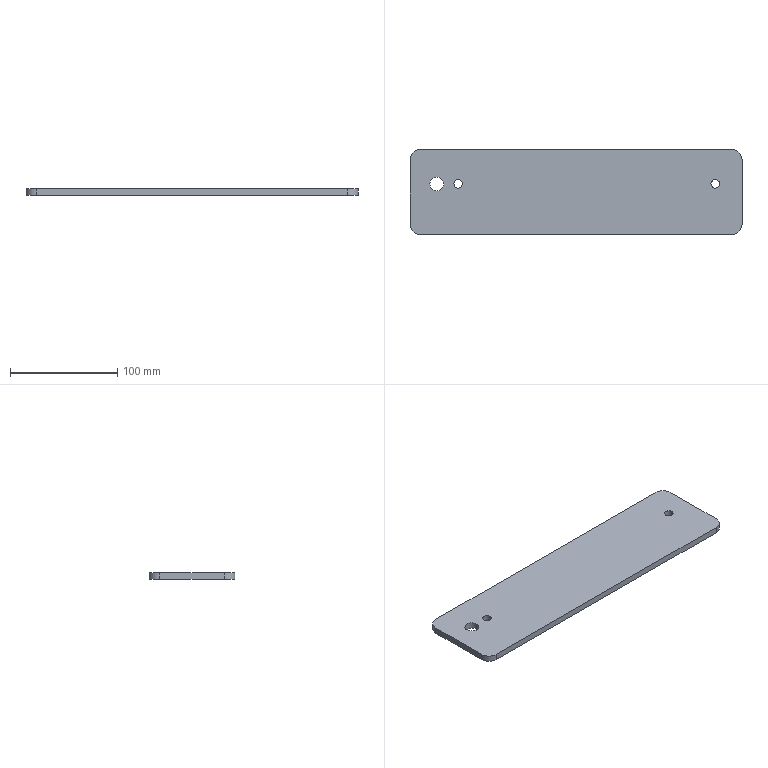Part | SolidWorks | features FlatPattern 1, SMBaseFlange 1, SheetMetal 1 | 1 solid | 16 faces | box 310 x 80 x 6 mm | volume 146885 mm3 | cylinder 10 | plane 6 | commonest cylinder face diameters 8 x4 20 x4 13 x2
STEP:
#1=CARTESIAN_POINT('',(-1194.,-927.5,6.));
#2=VERTEX_POINT('',#1);
#3=CARTESIAN_POINT('',(-1186.,-927.5,6.));
#4=VERTEX_POINT('',#3);
#5=CARTESIAN_POINT('',(-1190.,-927.5,6.));
#6=DIRECTION('',(0.,0.,1.));
#7=DIRECTION('',(1.,0.,0.));
#8=AXIS2_PLACEMENT_3D('',#5,#6,#7);
#9=CIRCLE('',#8,4.);
#10=EDGE_CURVE('',#2,#4,#9,.T.);
#11=ORIENTED_EDGE('',*,*,#10,.T.);
#12=CARTESIAN_POINT('',(-1186.,-927.5,0.));
#13=VERTEX_POINT('',#12);
#14=CARTESIAN_POINT('',(-1186.,-927.5,6.));
#15=DIRECTION('',(0.,0.,-1.));
#16=VECTOR('',#15,1000.);
#17=LINE('',#14,#16);
#18=EDGE_CURVE('',#4,#13,#17,.T.);
#19=ORIENTED_EDGE('',*,*,#18,.T.);
#20=CARTESIAN_POINT('',(-1194.,-927.5,0.));
#21=VERTEX_POINT('',#20);
#22=CARTESIAN_POINT('',(-1190.,-927.5,0.));
#23=DIRECTION('',(0.,0.,1.));
#24=DIRECTION('',(1.,0.,0.));
#25=AXIS2_PLACEMENT_3D('',#22,#23,#24);
#26=CIRCLE('',#25,4.);
#27=EDGE_CURVE('',#21,#13,#26,.T.);
#28=ORIENTED_EDGE('',*,*,#27,.F.);
#29=CARTESIAN_POINT('',(-1194.,-927.5,6.));
#30=DIRECTION('',(0.,0.,-1.));
#31=VECTOR('',#30,1000.);
#32=LINE('',#29,#31);
#33=EDGE_CURVE('',#2,#21,#32,.T.);
#34=ORIENTED_EDGE('',*,*,#33,.F.);
#35=EDGE_LOOP('',(#11,#19,#28,#34));
#36=FACE_OUTER_BOUND('',#35,.T.);
#37=CARTESIAN_POINT('',(-1190.,-927.5,6.));
#38=DIRECTION('',(0.,0.,-1.));
#39=DIRECTION('',(-1.,0.,0.));
#40=AXIS2_PLACEMENT_3D('',#37,#38,#39);
#41=CYLINDRICAL_SURFACE('',#40,4.);
#42=ADVANCED_FACE('',(#36),#41,.F.);
#43=CARTESIAN_POINT('',(-1434.,-927.5,6.));
#44=VERTEX_POINT('',#43);
#45=CARTESIAN_POINT('',(-1426.,-927.5,6.));
#46=VERTEX_POINT('',#45);
#47=CARTESIAN_POINT('',(-1430.,-927.5,6.));
#48=DIRECTION('',(0.,0.,1.));
#49=DIRECTION('',(1.,0.,0.));
#50=AXIS2_PLACEMENT_3D('',#47,#48,#49);
#51=CIRCLE('',#50,4.);
#52=EDGE_CURVE('',#44,#46,#51,.T.);
#53=ORIENTED_EDGE('',*,*,#52,.T.);
#54=CARTESIAN_POINT('',(-1426.,-927.5,0.));
#55=VERTEX_POINT('',#54);
#56=CARTESIAN_POINT('',(-1426.,-927.5,6.));
#57=DIRECTION('',(0.,0.,-1.));
#58=VECTOR('',#57,1000.);
#59=LINE('',#56,#58);
#60=EDGE_CURVE('',#46,#55,#59,.T.);
#61=ORIENTED_EDGE('',*,*,#60,.T.);
#62=CARTESIAN_POINT('',(-1434.,-927.5,0.));
#63=VERTEX_POINT('',#62);
#64=CARTESIAN_POINT('',(-1430.,-927.5,0.));
#65=DIRECTION('',(0.,0.,1.));
#66=DIRECTION('',(1.,0.,0.));
#67=AXIS2_PLACEMENT_3D('',#64,#65,#66);
#68=CIRCLE('',#67,4.);
#69=EDGE_CURVE('',#63,#55,#68,.T.);
#70=ORIENTED_EDGE('',*,*,#69,.F.);
#71=CARTESIAN_POINT('',(-1434.,-927.5,6.));
#72=DIRECTION('',(0.,0.,-1.));
#73=VECTOR('',#72,1000.);
#74=LINE('',#71,#73);
#75=EDGE_CURVE('',#44,#63,#74,.T.);
#76=ORIENTED_EDGE('',*,*,#75,.F.);
#77=EDGE_LOOP('',(#53,#61,#70,#76));
#78=FACE_OUTER_BOUND('',#77,.T.);
#79=CARTESIAN_POINT('',(-1430.,-927.5,6.));
#80=DIRECTION('',(0.,0.,-1.));
#81=DIRECTION('',(-1.,0.,0.));
#82=AXIS2_PLACEMENT_3D('',#79,#80,#81);
#83=CYLINDRICAL_SURFACE('',#82,4.);
#84=ADVANCED_FACE('',(#78),#83,.F.);
#85=CARTESIAN_POINT('',(-1456.5,-927.5,6.));
#86=VERTEX_POINT('',#85);
#87=CARTESIAN_POINT('',(-1443.5,-927.5,6.));
#88=VERTEX_POINT('',#87);
#89=CARTESIAN_POINT('',(-1450.,-927.5,6.));
#90=DIRECTION('',(0.,0.,1.));
#91=DIRECTION('',(1.,0.,0.));
#92=AXIS2_PLACEMENT_3D('',#89,#90,#91);
#93=CIRCLE('',#92,6.5);
#94=EDGE_CURVE('',#86,#88,#93,.T.);
#95=ORIENTED_EDGE('',*,*,#94,.T.);
#96=CARTESIAN_POINT('',(-1443.5,-927.5,0.));
#97=VERTEX_POINT('',#96);
#98=CARTESIAN_POINT('',(-1443.5,-927.5,6.));
#99=DIRECTION('',(0.,0.,-1.));
#100=VECTOR('',#99,1000.);
#101=LINE('',#98,#100);
#102=EDGE_CURVE('',#88,#97,#101,.T.);
#103=ORIENTED_EDGE('',*,*,#102,.T.);
#104=CARTESIAN_POINT('',(-1456.5,-927.5,0.));
#105=VERTEX_POINT('',#104);
#106=CARTESIAN_POINT('',(-1450.,-927.5,0.));
#107=DIRECTION('',(0.,0.,1.));
#108=DIRECTION('',(1.,0.,0.));
#109=AXIS2_PLACEMENT_3D('',#106,#107,#108);
#110=CIRCLE('',#109,6.5);
#111=EDGE_CURVE('',#105,#97,#110,.T.);
#112=ORIENTED_EDGE('',*,*,#111,.F.);
#113=CARTESIAN_POINT('',(-1456.5,-927.5,6.));
#114=DIRECTION('',(0.,0.,-1.));
#115=VECTOR('',#114,1000.);
#116=LINE('',#113,#115);
#117=EDGE_CURVE('',#86,#105,#116,.T.);
#118=ORIENTED_EDGE('',*,*,#117,.F.);
#119=EDGE_LOOP('',(#95,#103,#112,#118));
#120=FACE_OUTER_BOUND('',#119,.T.);
#121=CARTESIAN_POINT('',(-1450.,-927.5,6.));
#122=DIRECTION('',(0.,0.,-1.));
#123=DIRECTION('',(-1.,0.,0.));
#124=AXIS2_PLACEMENT_3D('',#121,#122,#123);
#125=CYLINDRICAL_SURFACE('',#124,6.5);
#126=ADVANCED_FACE('',(#120),#125,.F.);
#127=CARTESIAN_POINT('',(-1165.,-905.,6.));
#128=VERTEX_POINT('',#127);
#129=CARTESIAN_POINT('',(-1175.,-895.,6.));
#130=VERTEX_POINT('',#129);
#131=CARTESIAN_POINT('',(-1175.,-905.,6.));
#132=DIRECTION('',(0.,0.,1.));
#133=DIRECTION('',(-1.,0.,0.));
#134=AXIS2_PLACEMENT_3D('',#131,#132,#133);
#135=CIRCLE('',#134,10.);
#136=EDGE_CURVE('',#128,#130,#135,.T.);
#137=ORIENTED_EDGE('',*,*,#136,.T.);
#138=CARTESIAN_POINT('',(-1465.,-895.,6.));
#139=VERTEX_POINT('',#138);
#140=CARTESIAN_POINT('',(-1465.,-895.,6.));
#141=DIRECTION('',(-1.,0.,0.));
#142=VECTOR('',#141,1000.);
#143=LINE('',#140,#142);
#144=EDGE_CURVE('',#130,#139,#143,.T.);
#145=ORIENTED_EDGE('',*,*,#144,.T.);
#146=CARTESIAN_POINT('',(-1475.,-905.,6.));
#147=VERTEX_POINT('',#146);
#148=CARTESIAN_POINT('',(-1465.,-905.,6.));
#149=DIRECTION('',(0.,0.,1.));
#150=DIRECTION('',(-1.,0.,0.));
#151=AXIS2_PLACEMENT_3D('',#148,#149,#150);
#152=CIRCLE('',#151,10.);
#153=EDGE_CURVE('',#139,#147,#152,.T.);
#154=ORIENTED_EDGE('',*,*,#153,.T.);
#155=CARTESIAN_POINT('',(-1475.,-965.,6.));
#156=VERTEX_POINT('',#155);
#157=CARTESIAN_POINT('',(-1475.,-965.,6.));
#158=DIRECTION('',(0.,-1.,0.));
#159=VECTOR('',#158,1000.);
#160=LINE('',#157,#159);
#161=EDGE_CURVE('',#147,#156,#160,.T.);
#162=ORIENTED_EDGE('',*,*,#161,.T.);
#163=CARTESIAN_POINT('',(-1465.,-975.,6.));
#164=VERTEX_POINT('',#163);
#165=CARTESIAN_POINT('',(-1465.,-965.,6.));
#166=DIRECTION('',(0.,0.,1.));
#167=DIRECTION('',(-1.,0.,0.));
#168=AXIS2_PLACEMENT_3D('',#165,#166,#167);
#169=CIRCLE('',#168,10.);
#170=EDGE_CURVE('',#156,#164,#169,.T.);
#171=ORIENTED_EDGE('',*,*,#170,.T.);
#172=CARTESIAN_POINT('',(-1175.,-975.,6.));
#173=VERTEX_POINT('',#172);
#174=CARTESIAN_POINT('',(-1465.,-975.,6.));
#175=DIRECTION('',(1.,0.,0.));
#176=VECTOR('',#175,1000.);
#177=LINE('',#174,#176);
#178=EDGE_CURVE('',#164,#173,#177,.T.);
#179=ORIENTED_EDGE('',*,*,#178,.T.);
#180=CARTESIAN_POINT('',(-1165.,-965.,6.));
#181=VERTEX_POINT('',#180);
#182=CARTESIAN_POINT('',(-1175.,-965.,6.));
#183=DIRECTION('',(0.,0.,1.));
#184=DIRECTION('',(1.,0.,0.));
#185=AXIS2_PLACEMENT_3D('',#182,#183,#184);
#186=CIRCLE('',#185,10.);
#187=EDGE_CURVE('',#173,#181,#186,.T.);
#188=ORIENTED_EDGE('',*,*,#187,.T.);
#189=CARTESIAN_POINT('',(-1165.,-965.,6.));
#190=DIRECTION('',(0.,1.,0.));
#191=VECTOR('',#190,1000.);
#192=LINE('',#189,#191);
#193=EDGE_CURVE('',#181,#128,#192,.T.);
#194=ORIENTED_EDGE('',*,*,#193,.T.);
#195=EDGE_LOOP('',(#137,#145,#154,#162,#171,#179,#188,#194));
#196=FACE_OUTER_BOUND('',#195,.T.);
#197=ORIENTED_EDGE('',*,*,#94,.F.);
#198=CARTESIAN_POINT('',(-1450.,-927.5,6.));
#199=DIRECTION('',(0.,0.,1.));
#200=DIRECTION('',(1.,0.,0.));
#201=AXIS2_PLACEMENT_3D('',#198,#199,#200);
#202=CIRCLE('',#201,6.5);
#203=EDGE_CURVE('',#88,#86,#202,.T.);
#204=ORIENTED_EDGE('',*,*,#203,.F.);
#205=EDGE_LOOP('',(#197,#204));
#206=FACE_BOUND('',#205,.T.);
#207=ORIENTED_EDGE('',*,*,#52,.F.);
#208=CARTESIAN_POINT('',(-1430.,-927.5,6.));
#209=DIRECTION('',(0.,0.,1.));
#210=DIRECTION('',(1.,0.,0.));
#211=AXIS2_PLACEMENT_3D('',#208,#209,#210);
#212=CIRCLE('',#211,4.);
#213=EDGE_CURVE('',#46,#44,#212,.T.);
#214=ORIENTED_EDGE('',*,*,#213,.F.);
#215=EDGE_LOOP('',(#207,#214));
#216=FACE_BOUND('',#215,.T.);
#217=ORIENTED_EDGE('',*,*,#10,.F.);
#218=CARTESIAN_POINT('',(-1190.,-927.5,6.));
#219=DIRECTION('',(0.,0.,1.));
#220=DIRECTION('',(1.,0.,0.));
#221=AXIS2_PLACEMENT_3D('',#218,#219,#220);
#222=CIRCLE('',#221,4.);
#223=EDGE_CURVE('',#4,#2,#222,.T.);
#224=ORIENTED_EDGE('',*,*,#223,.F.);
#225=EDGE_LOOP('',(#217,#224));
#226=FACE_BOUND('',#225,.T.);
#227=CARTESIAN_POINT('',(-1175.,-905.,6.));
#228=DIRECTION('',(0.,0.,-1.));
#229=DIRECTION('',(-1.,0.,0.));
#230=AXIS2_PLACEMENT_3D('',#227,#228,#229);
#231=PLANE('',#230);
#232=ADVANCED_FACE('',(#196,#206,#216,#226),#231,.F.);
#233=ORIENTED_EDGE('',*,*,#69,.T.);
#234=CARTESIAN_POINT('',(-1430.,-927.5,0.));
#235=DIRECTION('',(0.,0.,1.));
#236=DIRECTION('',(1.,0.,0.));
#237=AXIS2_PLACEMENT_3D('',#234,#235,#236);
#238=CIRCLE('',#237,4.);
#239=EDGE_CURVE('',#55,#63,#238,.T.);
#240=ORIENTED_EDGE('',*,*,#239,.T.);
#241=EDGE_LOOP('',(#233,#240));
#242=FACE_BOUND('',#241,.T.);
#243=CARTESIAN_POINT('',(-1165.,-905.,0.));
#244=VERTEX_POINT('',#243);
#245=CARTESIAN_POINT('',(-1175.,-895.,0.));
#246=VERTEX_POINT('',#245);
#247=CARTESIAN_POINT('',(-1175.,-905.,0.));
#248=DIRECTION('',(0.,0.,1.));
#249=DIRECTION('',(-1.,0.,0.));
#250=AXIS2_PLACEMENT_3D('',#247,#248,#249);
#251=CIRCLE('',#250,10.);
#252=EDGE_CURVE('',#244,#246,#251,.T.);
#253=ORIENTED_EDGE('',*,*,#252,.F.);
#254=CARTESIAN_POINT('',(-1165.,-965.,0.));
#255=VERTEX_POINT('',#254);
#256=CARTESIAN_POINT('',(-1165.,-965.,0.));
#257=DIRECTION('',(0.,1.,0.));
#258=VECTOR('',#257,1000.);
#259=LINE('',#256,#258);
#260=EDGE_CURVE('',#255,#244,#259,.T.);
#261=ORIENTED_EDGE('',*,*,#260,.F.);
#262=CARTESIAN_POINT('',(-1175.,-975.,0.));
#263=VERTEX_POINT('',#262);
#264=CARTESIAN_POINT('',(-1175.,-965.,0.));
#265=DIRECTION('',(0.,0.,1.));
#266=DIRECTION('',(1.,0.,0.));
#267=AXIS2_PLACEMENT_3D('',#264,#265,#266);
#268=CIRCLE('',#267,10.);
#269=EDGE_CURVE('',#263,#255,#268,.T.);
#270=ORIENTED_EDGE('',*,*,#269,.F.);
#271=CARTESIAN_POINT('',(-1465.,-975.,0.));
#272=VERTEX_POINT('',#271);
#273=CARTESIAN_POINT('',(-1465.,-975.,0.));
#274=DIRECTION('',(1.,0.,0.));
#275=VECTOR('',#274,1000.);
#276=LINE('',#273,#275);
#277=EDGE_CURVE('',#272,#263,#276,.T.);
#278=ORIENTED_EDGE('',*,*,#277,.F.);
#279=CARTESIAN_POINT('',(-1475.,-965.,0.));
#280=VERTEX_POINT('',#279);
#281=CARTESIAN_POINT('',(-1465.,-965.,0.));
#282=DIRECTION('',(0.,0.,1.));
#283=DIRECTION('',(-1.,0.,0.));
#284=AXIS2_PLACEMENT_3D('',#281,#282,#283);
#285=CIRCLE('',#284,10.);
#286=EDGE_CURVE('',#280,#272,#285,.T.);
#287=ORIENTED_EDGE('',*,*,#286,.F.);
#288=CARTESIAN_POINT('',(-1475.,-905.,0.));
#289=VERTEX_POINT('',#288);
#290=CARTESIAN_POINT('',(-1475.,-965.,0.));
#291=DIRECTION('',(0.,-1.,0.));
#292=VECTOR('',#291,1000.);
#293=LINE('',#290,#292);
#294=EDGE_CURVE('',#289,#280,#293,.T.);
#295=ORIENTED_EDGE('',*,*,#294,.F.);
#296=CARTESIAN_POINT('',(-1465.,-895.,0.));
#297=VERTEX_POINT('',#296);
#298=CARTESIAN_POINT('',(-1465.,-905.,0.));
#299=DIRECTION('',(0.,0.,1.));
#300=DIRECTION('',(-1.,0.,0.));
#301=AXIS2_PLACEMENT_3D('',#298,#299,#300);
#302=CIRCLE('',#301,10.);
#303=EDGE_CURVE('',#297,#289,#302,.T.);
#304=ORIENTED_EDGE('',*,*,#303,.F.);
#305=CARTESIAN_POINT('',(-1465.,-895.,0.));
#306=DIRECTION('',(-1.,0.,0.));
#307=VECTOR('',#306,1000.);
#308=LINE('',#305,#307);
#309=EDGE_CURVE('',#246,#297,#308,.T.);
#310=ORIENTED_EDGE('',*,*,#309,.F.);
#311=EDGE_LOOP('',(#253,#261,#270,#278,#287,#295,#304,#310));
#312=FACE_OUTER_BOUND('',#311,.T.);
#313=ORIENTED_EDGE('',*,*,#111,.T.);
#314=CARTESIAN_POINT('',(-1450.,-927.5,0.));
#315=DIRECTION('',(0.,0.,1.));
#316=DIRECTION('',(1.,0.,0.));
#317=AXIS2_PLACEMENT_3D('',#314,#315,#316);
#318=CIRCLE('',#317,6.5);
#319=EDGE_CURVE('',#97,#105,#318,.T.);
#320=ORIENTED_EDGE('',*,*,#319,.T.);
#321=EDGE_LOOP('',(#313,#320));
#322=FACE_BOUND('',#321,.T.);
#323=ORIENTED_EDGE('',*,*,#27,.T.);
#324=CARTESIAN_POINT('',(-1190.,-927.5,0.));
#325=DIRECTION('',(0.,0.,1.));
#326=DIRECTION('',(1.,0.,0.));
#327=AXIS2_PLACEMENT_3D('',#324,#325,#326);
#328=CIRCLE('',#327,4.);
#329=EDGE_CURVE('',#13,#21,#328,.T.);
#330=ORIENTED_EDGE('',*,*,#329,.T.);
#331=EDGE_LOOP('',(#323,#330));
#332=FACE_BOUND('',#331,.T.);
#333=CARTESIAN_POINT('',(-1175.,-905.,0.));
#334=DIRECTION('',(0.,0.,-1.));
#335=DIRECTION('',(-1.,0.,0.));
#336=AXIS2_PLACEMENT_3D('',#333,#334,#335);
#337=PLANE('',#336);
#338=ADVANCED_FACE('',(#242,#312,#322,#332),#337,.T.);
#339=ORIENTED_EDGE('',*,*,#252,.T.);
#340=CARTESIAN_POINT('',(-1175.,-895.,6.));
#341=DIRECTION('',(0.,0.,-1.));
#342=VECTOR('',#341,1000.);
#343=LINE('',#340,#342);
#344=EDGE_CURVE('',#130,#246,#343,.T.);
#345=ORIENTED_EDGE('',*,*,#344,.F.);
#346=ORIENTED_EDGE('',*,*,#136,.F.);
#347=CARTESIAN_POINT('',(-1165.,-905.,6.));
#348=DIRECTION('',(0.,0.,-1.));
#349=VECTOR('',#348,1000.);
#350=LINE('',#347,#349);
#351=EDGE_CURVE('',#128,#244,#350,.T.);
#352=ORIENTED_EDGE('',*,*,#351,.T.);
#353=EDGE_LOOP('',(#339,#345,#346,#352));
#354=FACE_OUTER_BOUND('',#353,.T.);
#355=CARTESIAN_POINT('',(-1175.,-905.,6.));
#356=DIRECTION('',(0.,0.,-1.));
#357=DIRECTION('',(-1.,0.,0.));
#358=AXIS2_PLACEMENT_3D('',#355,#356,#357);
#359=CYLINDRICAL_SURFACE('',#358,10.);
#360=ADVANCED_FACE('',(#354),#359,.T.);
#361=ORIENTED_EDGE('',*,*,#309,.T.);
#362=CARTESIAN_POINT('',(-1465.,-895.,6.));
#363=DIRECTION('',(0.,0.,-1.));
#364=VECTOR('',#363,1000.);
#365=LINE('',#362,#364);
#366=EDGE_CURVE('',#139,#297,#365,.T.);
#367=ORIENTED_EDGE('',*,*,#366,.F.);
#368=ORIENTED_EDGE('',*,*,#144,.F.);
#369=ORIENTED_EDGE('',*,*,#344,.T.);
#370=EDGE_LOOP('',(#361,#367,#368,#369));
#371=FACE_OUTER_BOUND('',#370,.T.);
#372=CARTESIAN_POINT('',(-1465.,-895.,6.));
#373=DIRECTION('',(0.,-1.,0.));
#374=DIRECTION('',(0.,0.,-1.));
#375=AXIS2_PLACEMENT_3D('',#372,#373,#374);
#376=PLANE('',#375);
#377=ADVANCED_FACE('',(#371),#376,.F.);
#378=ORIENTED_EDGE('',*,*,#303,.T.);
#379=CARTESIAN_POINT('',(-1475.,-905.,6.));
#380=DIRECTION('',(0.,0.,-1.));
#381=VECTOR('',#380,1000.);
#382=LINE('',#379,#381);
#383=EDGE_CURVE('',#147,#289,#382,.T.);
#384=ORIENTED_EDGE('',*,*,#383,.F.);
#385=ORIENTED_EDGE('',*,*,#153,.F.);
#386=ORIENTED_EDGE('',*,*,#366,.T.);
#387=EDGE_LOOP('',(#378,#384,#385,#386));
#388=FACE_OUTER_BOUND('',#387,.T.);
#389=CARTESIAN_POINT('',(-1465.,-905.,6.));
#390=DIRECTION('',(0.,0.,-1.));
#391=DIRECTION('',(-1.,0.,0.));
#392=AXIS2_PLACEMENT_3D('',#389,#390,#391);
#393=CYLINDRICAL_SURFACE('',#392,10.);
#394=ADVANCED_FACE('',(#388),#393,.T.);
#395=ORIENTED_EDGE('',*,*,#294,.T.);
#396=CARTESIAN_POINT('',(-1475.,-965.,6.));
#397=DIRECTION('',(0.,0.,-1.));
#398=VECTOR('',#397,1000.);
#399=LINE('',#396,#398);
#400=EDGE_CURVE('',#156,#280,#399,.T.);
#401=ORIENTED_EDGE('',*,*,#400,.F.);
#402=ORIENTED_EDGE('',*,*,#161,.F.);
#403=ORIENTED_EDGE('',*,*,#383,.T.);
#404=EDGE_LOOP('',(#395,#401,#402,#403));
#405=FACE_OUTER_BOUND('',#404,.T.);
#406=CARTESIAN_POINT('',(-1475.,-965.,6.));
#407=DIRECTION('',(1.,0.,0.));
#408=DIRECTION('',(0.,0.,-1.));
#409=AXIS2_PLACEMENT_3D('',#406,#407,#408);
#410=PLANE('',#409);
#411=ADVANCED_FACE('',(#405),#410,.F.);
#412=ORIENTED_EDGE('',*,*,#286,.T.);
#413=CARTESIAN_POINT('',(-1465.,-975.,6.));
#414=DIRECTION('',(0.,0.,-1.));
#415=VECTOR('',#414,1000.);
#416=LINE('',#413,#415);
#417=EDGE_CURVE('',#164,#272,#416,.T.);
#418=ORIENTED_EDGE('',*,*,#417,.F.);
#419=ORIENTED_EDGE('',*,*,#170,.F.);
#420=ORIENTED_EDGE('',*,*,#400,.T.);
#421=EDGE_LOOP('',(#412,#418,#419,#420));
#422=FACE_OUTER_BOUND('',#421,.T.);
#423=CARTESIAN_POINT('',(-1465.,-965.,6.));
#424=DIRECTION('',(0.,0.,-1.));
#425=DIRECTION('',(-1.,0.,0.));
#426=AXIS2_PLACEMENT_3D('',#423,#424,#425);
#427=CYLINDRICAL_SURFACE('',#426,10.);
#428=ADVANCED_FACE('',(#422),#427,.T.);
#429=ORIENTED_EDGE('',*,*,#277,.T.);
#430=CARTESIAN_POINT('',(-1175.,-975.,6.));
#431=DIRECTION('',(0.,0.,-1.));
#432=VECTOR('',#431,1000.);
#433=LINE('',#430,#432);
#434=EDGE_CURVE('',#173,#263,#433,.T.);
#435=ORIENTED_EDGE('',*,*,#434,.F.);
#436=ORIENTED_EDGE('',*,*,#178,.F.);
#437=ORIENTED_EDGE('',*,*,#417,.T.);
#438=EDGE_LOOP('',(#429,#435,#436,#437));
#439=FACE_OUTER_BOUND('',#438,.T.);
#440=CARTESIAN_POINT('',(-1465.,-975.,6.));
#441=DIRECTION('',(0.,1.,0.));
#442=DIRECTION('',(0.,0.,1.));
#443=AXIS2_PLACEMENT_3D('',#440,#441,#442);
#444=PLANE('',#443);
#445=ADVANCED_FACE('',(#439),#444,.F.);
#446=ORIENTED_EDGE('',*,*,#269,.T.);
#447=CARTESIAN_POINT('',(-1165.,-965.,6.));
#448=DIRECTION('',(0.,0.,-1.));
#449=VECTOR('',#448,1000.);
#450=LINE('',#447,#449);
#451=EDGE_CURVE('',#181,#255,#450,.T.);
#452=ORIENTED_EDGE('',*,*,#451,.F.);
#453=ORIENTED_EDGE('',*,*,#187,.F.);
#454=ORIENTED_EDGE('',*,*,#434,.T.);
#455=EDGE_LOOP('',(#446,#452,#453,#454));
#456=FACE_OUTER_BOUND('',#455,.T.);
#457=CARTESIAN_POINT('',(-1175.,-965.,6.));
#458=DIRECTION('',(0.,0.,-1.));
#459=DIRECTION('',(-1.,0.,0.));
#460=AXIS2_PLACEMENT_3D('',#457,#458,#459);
#461=CYLINDRICAL_SURFACE('',#460,10.);
#462=ADVANCED_FACE('',(#456),#461,.T.);
#463=ORIENTED_EDGE('',*,*,#260,.T.);
#464=ORIENTED_EDGE('',*,*,#351,.F.);
#465=ORIENTED_EDGE('',*,*,#193,.F.);
#466=ORIENTED_EDGE('',*,*,#451,.T.);
#467=EDGE_LOOP('',(#463,#464,#465,#466));
#468=FACE_OUTER_BOUND('',#467,.T.);
#469=CARTESIAN_POINT('',(-1165.,-965.,6.));
#470=DIRECTION('',(-1.,0.,0.));
#471=DIRECTION('',(0.,0.,1.));
#472=AXIS2_PLACEMENT_3D('',#469,#470,#471);
#473=PLANE('',#472);
#474=ADVANCED_FACE('',(#468),#473,.F.);
#475=ORIENTED_EDGE('',*,*,#102,.F.);
#476=ORIENTED_EDGE('',*,*,#203,.T.);
#477=ORIENTED_EDGE('',*,*,#117,.T.);
#478=ORIENTED_EDGE('',*,*,#319,.F.);
#479=EDGE_LOOP('',(#475,#476,#477,#478));
#480=FACE_OUTER_BOUND('',#479,.T.);
#481=CARTESIAN_POINT('',(-1450.,-927.5,6.));
#482=DIRECTION('',(0.,0.,-1.));
#483=DIRECTION('',(-1.,0.,0.));
#484=AXIS2_PLACEMENT_3D('',#481,#482,#483);
#485=CYLINDRICAL_SURFACE('',#484,6.5);
#486=ADVANCED_FACE('',(#480),#485,.F.);
#487=ORIENTED_EDGE('',*,*,#60,.F.);
#488=ORIENTED_EDGE('',*,*,#213,.T.);
#489=ORIENTED_EDGE('',*,*,#75,.T.);
#490=ORIENTED_EDGE('',*,*,#239,.F.);
#491=EDGE_LOOP('',(#487,#488,#489,#490));
#492=FACE_OUTER_BOUND('',#491,.T.);
#493=CARTESIAN_POINT('',(-1430.,-927.5,6.));
#494=DIRECTION('',(0.,0.,-1.));
#495=DIRECTION('',(-1.,0.,0.));
#496=AXIS2_PLACEMENT_3D('',#493,#494,#495);
#497=CYLINDRICAL_SURFACE('',#496,4.);
#498=ADVANCED_FACE('',(#492),#497,.F.);
#499=ORIENTED_EDGE('',*,*,#18,.F.);
#500=ORIENTED_EDGE('',*,*,#223,.T.);
#501=ORIENTED_EDGE('',*,*,#33,.T.);
#502=ORIENTED_EDGE('',*,*,#329,.F.);
#503=EDGE_LOOP('',(#499,#500,#501,#502));
#504=FACE_OUTER_BOUND('',#503,.T.);
#505=CARTESIAN_POINT('',(-1190.,-927.5,6.));
#506=DIRECTION('',(0.,0.,-1.));
#507=DIRECTION('',(-1.,0.,0.));
#508=AXIS2_PLACEMENT_3D('',#505,#506,#507);
#509=CYLINDRICAL_SURFACE('',#508,4.);
#510=ADVANCED_FACE('',(#504),#509,.F.);
#511=CLOSED_SHELL('',(#42,#84,#126,#232,#338,#360,#377,#394,#411,#428,#445,#462,#474,#486,#498,#510));
#512=MANIFOLD_SOLID_BREP('',#511);
#513=CARTESIAN_POINT('',(0.,0.,0.));
#514=DIRECTION('',(0.,0.,1.));
#515=DIRECTION('',(1.,0.,0.));
#516=AXIS2_PLACEMENT_3D('',#513,#514,#515);
#517=(LENGTH_UNIT()NAMED_UNIT(*)SI_UNIT(.MILLI.,.METRE.));
#518=UNCERTAINTY_MEASURE_WITH_UNIT(LENGTH_MEASURE(0.00001),#517,'','');
#519=(NAMED_UNIT(*)PLANE_ANGLE_UNIT()SI_UNIT($,.RADIAN.));
#520=(NAMED_UNIT(*)SI_UNIT($,.STERADIAN.)SOLID_ANGLE_UNIT());
#521=(GEOMETRIC_REPRESENTATION_CONTEXT(3)GLOBAL_UNCERTAINTY_ASSIGNED_CONTEXT((#518))GLOBAL_UNIT_ASSIGNED_CONTEXT((#517,#519,#520))REPRESENTATION_CONTEXT('',''));
#522=ADVANCED_BREP_SHAPE_REPRESENTATION('',(#512,#516),#521);